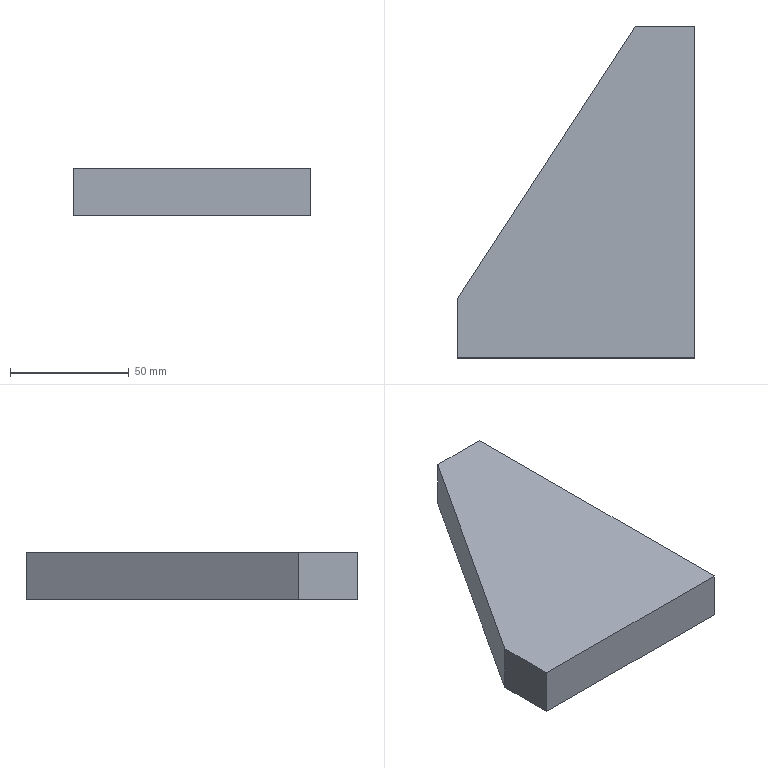Part | SolidWorks | features Extrusion 1 | 1 solid | 7 faces | box 100 x 140 x 20 mm | volume 193750 mm3 | plane 7
STEP:
#1=CARTESIAN_POINT('',(0.,25.,0.));
#2=VERTEX_POINT('',#1);
#3=CARTESIAN_POINT('',(0.,0.,0.));
#4=VERTEX_POINT('',#3);
#5=CARTESIAN_POINT('',(0.,25.,0.));
#6=DIRECTION('',(0.,-1.,0.));
#7=VECTOR('',#6,1000.);
#8=LINE('',#5,#7);
#9=EDGE_CURVE('',#2,#4,#8,.T.);
#10=ORIENTED_EDGE('',*,*,#9,.T.);
#11=CARTESIAN_POINT('',(0.,0.,20.));
#12=VERTEX_POINT('',#11);
#13=CARTESIAN_POINT('',(0.,0.,20.));
#14=DIRECTION('',(0.,0.,-1.));
#15=VECTOR('',#14,1000.);
#16=LINE('',#13,#15);
#17=EDGE_CURVE('',#12,#4,#16,.T.);
#18=ORIENTED_EDGE('',*,*,#17,.F.);
#19=CARTESIAN_POINT('',(0.,25.,20.));
#20=VERTEX_POINT('',#19);
#21=CARTESIAN_POINT('',(0.,25.,20.));
#22=DIRECTION('',(0.,-1.,0.));
#23=VECTOR('',#22,1000.);
#24=LINE('',#21,#23);
#25=EDGE_CURVE('',#20,#12,#24,.T.);
#26=ORIENTED_EDGE('',*,*,#25,.F.);
#27=CARTESIAN_POINT('',(0.,25.,20.));
#28=DIRECTION('',(0.,0.,-1.));
#29=VECTOR('',#28,1000.);
#30=LINE('',#27,#29);
#31=EDGE_CURVE('',#20,#2,#30,.T.);
#32=ORIENTED_EDGE('',*,*,#31,.T.);
#33=EDGE_LOOP('',(#10,#18,#26,#32));
#34=FACE_OUTER_BOUND('',#33,.T.);
#35=CARTESIAN_POINT('',(0.,25.,20.));
#36=DIRECTION('',(1.,0.,0.));
#37=DIRECTION('',(0.,1.,0.));
#38=AXIS2_PLACEMENT_3D('',#35,#36,#37);
#39=PLANE('',#38);
#40=ADVANCED_FACE('',(#34),#39,.F.);
#41=CARTESIAN_POINT('',(100.,0.,0.));
#42=VERTEX_POINT('',#41);
#43=CARTESIAN_POINT('',(0.,0.,0.));
#44=DIRECTION('',(1.,0.,0.));
#45=VECTOR('',#44,1000.);
#46=LINE('',#43,#45);
#47=EDGE_CURVE('',#4,#42,#46,.T.);
#48=ORIENTED_EDGE('',*,*,#47,.T.);
#49=CARTESIAN_POINT('',(100.,0.,20.));
#50=VERTEX_POINT('',#49);
#51=CARTESIAN_POINT('',(100.,0.,20.));
#52=DIRECTION('',(0.,0.,-1.));
#53=VECTOR('',#52,1000.);
#54=LINE('',#51,#53);
#55=EDGE_CURVE('',#50,#42,#54,.T.);
#56=ORIENTED_EDGE('',*,*,#55,.F.);
#57=CARTESIAN_POINT('',(0.,0.,20.));
#58=DIRECTION('',(1.,0.,0.));
#59=VECTOR('',#58,1000.);
#60=LINE('',#57,#59);
#61=EDGE_CURVE('',#12,#50,#60,.T.);
#62=ORIENTED_EDGE('',*,*,#61,.F.);
#63=ORIENTED_EDGE('',*,*,#17,.T.);
#64=EDGE_LOOP('',(#48,#56,#62,#63));
#65=FACE_OUTER_BOUND('',#64,.T.);
#66=CARTESIAN_POINT('',(0.,0.,20.));
#67=DIRECTION('',(0.,1.,0.));
#68=DIRECTION('',(0.,0.,1.));
#69=AXIS2_PLACEMENT_3D('',#66,#67,#68);
#70=PLANE('',#69);
#71=ADVANCED_FACE('',(#65),#70,.F.);
#72=CARTESIAN_POINT('',(100.,140.,0.));
#73=VERTEX_POINT('',#72);
#74=CARTESIAN_POINT('',(100.,0.,0.));
#75=DIRECTION('',(0.,1.,0.));
#76=VECTOR('',#75,1000.);
#77=LINE('',#74,#76);
#78=EDGE_CURVE('',#42,#73,#77,.T.);
#79=ORIENTED_EDGE('',*,*,#78,.T.);
#80=CARTESIAN_POINT('',(100.,140.,20.));
#81=VERTEX_POINT('',#80);
#82=CARTESIAN_POINT('',(100.,140.,20.));
#83=DIRECTION('',(0.,0.,-1.));
#84=VECTOR('',#83,1000.);
#85=LINE('',#82,#84);
#86=EDGE_CURVE('',#81,#73,#85,.T.);
#87=ORIENTED_EDGE('',*,*,#86,.F.);
#88=CARTESIAN_POINT('',(100.,0.,20.));
#89=DIRECTION('',(0.,1.,0.));
#90=VECTOR('',#89,1000.);
#91=LINE('',#88,#90);
#92=EDGE_CURVE('',#50,#81,#91,.T.);
#93=ORIENTED_EDGE('',*,*,#92,.F.);
#94=ORIENTED_EDGE('',*,*,#55,.T.);
#95=EDGE_LOOP('',(#79,#87,#93,#94));
#96=FACE_OUTER_BOUND('',#95,.T.);
#97=CARTESIAN_POINT('',(100.,0.,20.));
#98=DIRECTION('',(-1.,0.,0.));
#99=DIRECTION('',(0.,0.,1.));
#100=AXIS2_PLACEMENT_3D('',#97,#98,#99);
#101=PLANE('',#100);
#102=ADVANCED_FACE('',(#96),#101,.F.);
#103=CARTESIAN_POINT('',(75.,140.,0.));
#104=VERTEX_POINT('',#103);
#105=CARTESIAN_POINT('',(100.,140.,0.));
#106=DIRECTION('',(-1.,0.,0.));
#107=VECTOR('',#106,1000.);
#108=LINE('',#105,#107);
#109=EDGE_CURVE('',#73,#104,#108,.T.);
#110=ORIENTED_EDGE('',*,*,#109,.T.);
#111=CARTESIAN_POINT('',(75.,140.,20.));
#112=VERTEX_POINT('',#111);
#113=CARTESIAN_POINT('',(75.,140.,20.));
#114=DIRECTION('',(0.,0.,-1.));
#115=VECTOR('',#114,1000.);
#116=LINE('',#113,#115);
#117=EDGE_CURVE('',#112,#104,#116,.T.);
#118=ORIENTED_EDGE('',*,*,#117,.F.);
#119=CARTESIAN_POINT('',(100.,140.,20.));
#120=DIRECTION('',(-1.,0.,0.));
#121=VECTOR('',#120,1000.);
#122=LINE('',#119,#121);
#123=EDGE_CURVE('',#81,#112,#122,.T.);
#124=ORIENTED_EDGE('',*,*,#123,.F.);
#125=ORIENTED_EDGE('',*,*,#86,.T.);
#126=EDGE_LOOP('',(#110,#118,#124,#125));
#127=FACE_OUTER_BOUND('',#126,.T.);
#128=CARTESIAN_POINT('',(100.,140.,20.));
#129=DIRECTION('',(0.,-1.,0.));
#130=DIRECTION('',(0.,0.,-1.));
#131=AXIS2_PLACEMENT_3D('',#128,#129,#130);
#132=PLANE('',#131);
#133=ADVANCED_FACE('',(#127),#132,.F.);
#134=CARTESIAN_POINT('',(75.,140.,0.));
#135=DIRECTION('',(-0.5463,-0.8376,0.));
#136=VECTOR('',#135,1000.);
#137=LINE('',#134,#136);
#138=EDGE_CURVE('',#104,#2,#137,.T.);
#139=ORIENTED_EDGE('',*,*,#138,.T.);
#140=ORIENTED_EDGE('',*,*,#31,.F.);
#141=CARTESIAN_POINT('',(75.,140.,20.));
#142=DIRECTION('',(-0.5463,-0.8376,0.));
#143=VECTOR('',#142,1000.);
#144=LINE('',#141,#143);
#145=EDGE_CURVE('',#112,#20,#144,.T.);
#146=ORIENTED_EDGE('',*,*,#145,.F.);
#147=ORIENTED_EDGE('',*,*,#117,.T.);
#148=EDGE_LOOP('',(#139,#140,#146,#147));
#149=FACE_OUTER_BOUND('',#148,.T.);
#150=CARTESIAN_POINT('',(75.,140.,20.));
#151=DIRECTION('',(0.8376,-0.5463,0.));
#152=DIRECTION('',(0.5463,0.8376,0.));
#153=AXIS2_PLACEMENT_3D('',#150,#151,#152);
#154=PLANE('',#153);
#155=ADVANCED_FACE('',(#149),#154,.F.);
#156=ORIENTED_EDGE('',*,*,#25,.T.);
#157=ORIENTED_EDGE('',*,*,#61,.T.);
#158=ORIENTED_EDGE('',*,*,#92,.T.);
#159=ORIENTED_EDGE('',*,*,#123,.T.);
#160=ORIENTED_EDGE('',*,*,#145,.T.);
#161=EDGE_LOOP('',(#156,#157,#158,#159,#160));
#162=FACE_OUTER_BOUND('',#161,.T.);
#163=CARTESIAN_POINT('',(0.,0.,20.));
#164=DIRECTION('',(0.,0.,1.));
#165=DIRECTION('',(1.,0.,0.));
#166=AXIS2_PLACEMENT_3D('',#163,#164,#165);
#167=PLANE('',#166);
#168=ADVANCED_FACE('',(#162),#167,.T.);
#169=ORIENTED_EDGE('',*,*,#9,.F.);
#170=ORIENTED_EDGE('',*,*,#138,.F.);
#171=ORIENTED_EDGE('',*,*,#109,.F.);
#172=ORIENTED_EDGE('',*,*,#78,.F.);
#173=ORIENTED_EDGE('',*,*,#47,.F.);
#174=EDGE_LOOP('',(#169,#170,#171,#172,#173));
#175=FACE_OUTER_BOUND('',#174,.T.);
#176=CARTESIAN_POINT('',(0.,0.,0.));
#177=DIRECTION('',(0.,0.,1.));
#178=DIRECTION('',(1.,0.,0.));
#179=AXIS2_PLACEMENT_3D('',#176,#177,#178);
#180=PLANE('',#179);
#181=ADVANCED_FACE('',(#175),#180,.F.);
#182=CLOSED_SHELL('',(#40,#71,#102,#133,#155,#168,#181));
#183=MANIFOLD_SOLID_BREP('',#182);
#184=CARTESIAN_POINT('',(0.,0.,0.));
#185=DIRECTION('',(0.,0.,1.));
#186=DIRECTION('',(1.,0.,0.));
#187=AXIS2_PLACEMENT_3D('',#184,#185,#186);
#188=(LENGTH_UNIT()NAMED_UNIT(*)SI_UNIT(.MILLI.,.METRE.));
#189=UNCERTAINTY_MEASURE_WITH_UNIT(LENGTH_MEASURE(0.00001),#188,'','');
#190=(NAMED_UNIT(*)PLANE_ANGLE_UNIT()SI_UNIT($,.RADIAN.));
#191=(NAMED_UNIT(*)SI_UNIT($,.STERADIAN.)SOLID_ANGLE_UNIT());
#192=(GEOMETRIC_REPRESENTATION_CONTEXT(3)GLOBAL_UNCERTAINTY_ASSIGNED_CONTEXT((#189))GLOBAL_UNIT_ASSIGNED_CONTEXT((#188,#190,#191))REPRESENTATION_CONTEXT('',''));
#193=ADVANCED_BREP_SHAPE_REPRESENTATION('',(#183,#187),#192);